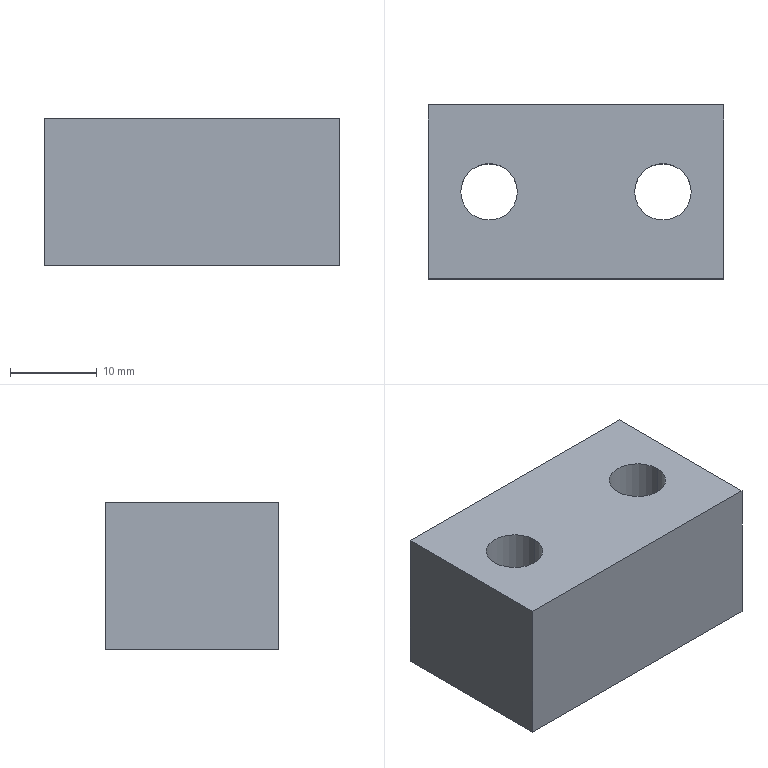Part | STEP file | push magnet seat spacer block 1 | 1 solid | 10 faces | box 34 x 20 x 17 mm | volume 10432 mm3 | plane 6 | cylinder 4 | commonest cylinder face diameters 6.5 x4
STEP:
#1=CARTESIAN_POINT('',(0.,0.,0.));
#2=DIRECTION('',(0.,0.,1.));
#3=DIRECTION('',(1.,0.,0.));
#4=AXIS2_PLACEMENT_3D('',#1,#2,#3);
#5=CARTESIAN_POINT('',(-13.25,0.,17.));
#6=VERTEX_POINT('',#5);
#7=CARTESIAN_POINT('',(-13.25,0.,0.));
#8=VERTEX_POINT('',#7);
#9=CARTESIAN_POINT('',(-13.25,0.,17.));
#10=DIRECTION('',(0.,0.,-1.));
#11=VECTOR('',#10,1.);
#12=LINE('',#9,#11);
#13=CARTESIAN_POINT('',(-10.,0.,17.));
#14=DIRECTION('',(0.,0.,-1.));
#15=DIRECTION('',(-1.,0.,0.));
#16=AXIS2_PLACEMENT_3D('',#13,#14,#15);
#17=CYLINDRICAL_SURFACE('',#16,3.25);
#18=CARTESIAN_POINT('',(6.283,0.));
#19=DIRECTION('',(0.,1.));
#20=VECTOR('',#19,1.);
#21=LINE('',#18,#20);
#22=(GEOMETRIC_REPRESENTATION_CONTEXT(2)PARAMETRIC_REPRESENTATION_CONTEXT()REPRESENTATION_CONTEXT('',''));
#23=DEFINITIONAL_REPRESENTATION('',(#21),#22);
#24=PCURVE('',#17,#23);
#25=CARTESIAN_POINT('',(-10.,0.,17.));
#26=DIRECTION('',(0.,0.,-1.));
#27=DIRECTION('',(-1.,0.,0.));
#28=AXIS2_PLACEMENT_3D('',#25,#26,#27);
#29=CYLINDRICAL_SURFACE('',#28,3.25);
#30=CARTESIAN_POINT('',(0.,0.));
#31=DIRECTION('',(0.,1.));
#32=VECTOR('',#31,1.);
#33=LINE('',#30,#32);
#34=(GEOMETRIC_REPRESENTATION_CONTEXT(2)PARAMETRIC_REPRESENTATION_CONTEXT()REPRESENTATION_CONTEXT('',''));
#35=DEFINITIONAL_REPRESENTATION('',(#33),#34);
#36=PCURVE('',#29,#35);
#37=SURFACE_CURVE('',#12,(#24,#36),.PCURVE_S1.);
#38=EDGE_CURVE('',#6,#8,#37,.T.);
#39=ORIENTED_EDGE('',*,*,#38,.T.);
#40=CARTESIAN_POINT('',(-6.75,0.,0.));
#41=VERTEX_POINT('',#40);
#42=CARTESIAN_POINT('',(-10.,0.,0.));
#43=DIRECTION('',(0.,0.,1.));
#44=DIRECTION('',(1.,0.,0.));
#45=AXIS2_PLACEMENT_3D('',#42,#43,#44);
#46=CIRCLE('',#45,3.25);
#47=CARTESIAN_POINT('',(9.425,17.));
#48=DIRECTION('',(-1.,0.));
#49=VECTOR('',#48,1.);
#50=LINE('',#47,#49);
#51=(GEOMETRIC_REPRESENTATION_CONTEXT(2)PARAMETRIC_REPRESENTATION_CONTEXT()REPRESENTATION_CONTEXT('',''));
#52=DEFINITIONAL_REPRESENTATION('',(#50),#51);
#53=PCURVE('',#17,#52);
#54=CARTESIAN_POINT('',(17.,-10.,0.));
#55=DIRECTION('',(0.,0.,1.));
#56=DIRECTION('',(1.,0.,0.));
#57=AXIS2_PLACEMENT_3D('',#54,#55,#56);
#58=PLANE('',#57);
#59=CARTESIAN_POINT('',(-27.,10.));
#60=DIRECTION('',(1.,0.));
#61=AXIS2_PLACEMENT_2D('',#59,#60);
#62=CIRCLE('',#61,3.25);
#63=(GEOMETRIC_REPRESENTATION_CONTEXT(2)PARAMETRIC_REPRESENTATION_CONTEXT()REPRESENTATION_CONTEXT('',''));
#64=DEFINITIONAL_REPRESENTATION('',(#62),#63);
#65=PCURVE('',#58,#64);
#66=SURFACE_CURVE('',#46,(#53,#65),.PCURVE_S1.);
#67=EDGE_CURVE('',#8,#41,#66,.T.);
#68=ORIENTED_EDGE('',*,*,#67,.T.);
#69=CARTESIAN_POINT('',(-6.75,0.,17.));
#70=VERTEX_POINT('',#69);
#71=CARTESIAN_POINT('',(-6.75,0.,17.));
#72=DIRECTION('',(0.,0.,-1.));
#73=VECTOR('',#72,1.);
#74=LINE('',#71,#73);
#75=CARTESIAN_POINT('',(3.142,0.));
#76=DIRECTION('',(0.,1.));
#77=VECTOR('',#76,1.);
#78=LINE('',#75,#77);
#79=(GEOMETRIC_REPRESENTATION_CONTEXT(2)PARAMETRIC_REPRESENTATION_CONTEXT()REPRESENTATION_CONTEXT('',''));
#80=DEFINITIONAL_REPRESENTATION('',(#78),#79);
#81=PCURVE('',#17,#80);
#82=CARTESIAN_POINT('',(3.142,0.));
#83=DIRECTION('',(0.,1.));
#84=VECTOR('',#83,1.);
#85=LINE('',#82,#84);
#86=(GEOMETRIC_REPRESENTATION_CONTEXT(2)PARAMETRIC_REPRESENTATION_CONTEXT()REPRESENTATION_CONTEXT('',''));
#87=DEFINITIONAL_REPRESENTATION('',(#85),#86);
#88=PCURVE('',#29,#87);
#89=SURFACE_CURVE('',#74,(#81,#88),.PCURVE_S1.);
#90=EDGE_CURVE('',#70,#41,#89,.T.);
#91=ORIENTED_EDGE('',*,*,#90,.F.);
#92=CARTESIAN_POINT('',(-10.,0.,17.));
#93=DIRECTION('',(0.,0.,1.));
#94=DIRECTION('',(1.,0.,0.));
#95=AXIS2_PLACEMENT_3D('',#92,#93,#94);
#96=CIRCLE('',#95,3.25);
#97=CARTESIAN_POINT('',(9.425,0.));
#98=DIRECTION('',(-1.,0.));
#99=VECTOR('',#98,1.);
#100=LINE('',#97,#99);
#101=(GEOMETRIC_REPRESENTATION_CONTEXT(2)PARAMETRIC_REPRESENTATION_CONTEXT()REPRESENTATION_CONTEXT('',''));
#102=DEFINITIONAL_REPRESENTATION('',(#100),#101);
#103=PCURVE('',#17,#102);
#104=CARTESIAN_POINT('',(17.,-10.,17.));
#105=DIRECTION('',(0.,0.,1.));
#106=DIRECTION('',(1.,0.,0.));
#107=AXIS2_PLACEMENT_3D('',#104,#105,#106);
#108=PLANE('',#107);
#109=CARTESIAN_POINT('',(-27.,10.));
#110=DIRECTION('',(1.,0.));
#111=AXIS2_PLACEMENT_2D('',#109,#110);
#112=CIRCLE('',#111,3.25);
#113=(GEOMETRIC_REPRESENTATION_CONTEXT(2)PARAMETRIC_REPRESENTATION_CONTEXT()REPRESENTATION_CONTEXT('',''));
#114=DEFINITIONAL_REPRESENTATION('',(#112),#113);
#115=PCURVE('',#108,#114);
#116=SURFACE_CURVE('',#96,(#103,#115),.PCURVE_S1.);
#117=EDGE_CURVE('',#6,#70,#116,.T.);
#118=ORIENTED_EDGE('',*,*,#117,.F.);
#119=EDGE_LOOP('',(#39,#68,#91,#118));
#120=FACE_BOUND('',#119,.F.);
#121=ADVANCED_FACE('',(#120),#17,.F.);
#122=CARTESIAN_POINT('',(6.75,0.,17.));
#123=VERTEX_POINT('',#122);
#124=CARTESIAN_POINT('',(6.75,0.,0.));
#125=VERTEX_POINT('',#124);
#126=CARTESIAN_POINT('',(6.75,0.,17.));
#127=DIRECTION('',(0.,0.,-1.));
#128=VECTOR('',#127,1.);
#129=LINE('',#126,#128);
#130=CARTESIAN_POINT('',(10.,0.,17.));
#131=DIRECTION('',(0.,0.,-1.));
#132=DIRECTION('',(-1.,0.,0.));
#133=AXIS2_PLACEMENT_3D('',#130,#131,#132);
#134=CYLINDRICAL_SURFACE('',#133,3.25);
#135=CARTESIAN_POINT('',(6.283,0.));
#136=DIRECTION('',(0.,1.));
#137=VECTOR('',#136,1.);
#138=LINE('',#135,#137);
#139=(GEOMETRIC_REPRESENTATION_CONTEXT(2)PARAMETRIC_REPRESENTATION_CONTEXT()REPRESENTATION_CONTEXT('',''));
#140=DEFINITIONAL_REPRESENTATION('',(#138),#139);
#141=PCURVE('',#134,#140);
#142=CARTESIAN_POINT('',(10.,0.,17.));
#143=DIRECTION('',(0.,0.,-1.));
#144=DIRECTION('',(-1.,0.,0.));
#145=AXIS2_PLACEMENT_3D('',#142,#143,#144);
#146=CYLINDRICAL_SURFACE('',#145,3.25);
#147=CARTESIAN_POINT('',(0.,0.));
#148=DIRECTION('',(0.,1.));
#149=VECTOR('',#148,1.);
#150=LINE('',#147,#149);
#151=(GEOMETRIC_REPRESENTATION_CONTEXT(2)PARAMETRIC_REPRESENTATION_CONTEXT()REPRESENTATION_CONTEXT('',''));
#152=DEFINITIONAL_REPRESENTATION('',(#150),#151);
#153=PCURVE('',#146,#152);
#154=SURFACE_CURVE('',#129,(#141,#153),.PCURVE_S1.);
#155=EDGE_CURVE('',#123,#125,#154,.T.);
#156=ORIENTED_EDGE('',*,*,#155,.T.);
#157=CARTESIAN_POINT('',(13.25,0.,0.));
#158=VERTEX_POINT('',#157);
#159=CARTESIAN_POINT('',(10.,0.,0.));
#160=DIRECTION('',(0.,0.,1.));
#161=DIRECTION('',(1.,0.,0.));
#162=AXIS2_PLACEMENT_3D('',#159,#160,#161);
#163=CIRCLE('',#162,3.25);
#164=CARTESIAN_POINT('',(9.425,17.));
#165=DIRECTION('',(-1.,0.));
#166=VECTOR('',#165,1.);
#167=LINE('',#164,#166);
#168=(GEOMETRIC_REPRESENTATION_CONTEXT(2)PARAMETRIC_REPRESENTATION_CONTEXT()REPRESENTATION_CONTEXT('',''));
#169=DEFINITIONAL_REPRESENTATION('',(#167),#168);
#170=PCURVE('',#134,#169);
#171=CARTESIAN_POINT('',(-7.,10.));
#172=DIRECTION('',(1.,0.));
#173=AXIS2_PLACEMENT_2D('',#171,#172);
#174=CIRCLE('',#173,3.25);
#175=(GEOMETRIC_REPRESENTATION_CONTEXT(2)PARAMETRIC_REPRESENTATION_CONTEXT()REPRESENTATION_CONTEXT('',''));
#176=DEFINITIONAL_REPRESENTATION('',(#174),#175);
#177=PCURVE('',#58,#176);
#178=SURFACE_CURVE('',#163,(#170,#177),.PCURVE_S1.);
#179=EDGE_CURVE('',#125,#158,#178,.T.);
#180=ORIENTED_EDGE('',*,*,#179,.T.);
#181=CARTESIAN_POINT('',(13.25,0.,17.));
#182=VERTEX_POINT('',#181);
#183=CARTESIAN_POINT('',(13.25,0.,17.));
#184=DIRECTION('',(0.,0.,-1.));
#185=VECTOR('',#184,1.);
#186=LINE('',#183,#185);
#187=CARTESIAN_POINT('',(3.142,0.));
#188=DIRECTION('',(0.,1.));
#189=VECTOR('',#188,1.);
#190=LINE('',#187,#189);
#191=(GEOMETRIC_REPRESENTATION_CONTEXT(2)PARAMETRIC_REPRESENTATION_CONTEXT()REPRESENTATION_CONTEXT('',''));
#192=DEFINITIONAL_REPRESENTATION('',(#190),#191);
#193=PCURVE('',#134,#192);
#194=CARTESIAN_POINT('',(3.142,0.));
#195=DIRECTION('',(0.,1.));
#196=VECTOR('',#195,1.);
#197=LINE('',#194,#196);
#198=(GEOMETRIC_REPRESENTATION_CONTEXT(2)PARAMETRIC_REPRESENTATION_CONTEXT()REPRESENTATION_CONTEXT('',''));
#199=DEFINITIONAL_REPRESENTATION('',(#197),#198);
#200=PCURVE('',#146,#199);
#201=SURFACE_CURVE('',#186,(#193,#200),.PCURVE_S1.);
#202=EDGE_CURVE('',#182,#158,#201,.T.);
#203=ORIENTED_EDGE('',*,*,#202,.F.);
#204=CARTESIAN_POINT('',(10.,0.,17.));
#205=DIRECTION('',(0.,0.,1.));
#206=DIRECTION('',(1.,0.,0.));
#207=AXIS2_PLACEMENT_3D('',#204,#205,#206);
#208=CIRCLE('',#207,3.25);
#209=CARTESIAN_POINT('',(9.425,0.));
#210=DIRECTION('',(-1.,0.));
#211=VECTOR('',#210,1.);
#212=LINE('',#209,#211);
#213=(GEOMETRIC_REPRESENTATION_CONTEXT(2)PARAMETRIC_REPRESENTATION_CONTEXT()REPRESENTATION_CONTEXT('',''));
#214=DEFINITIONAL_REPRESENTATION('',(#212),#213);
#215=PCURVE('',#134,#214);
#216=CARTESIAN_POINT('',(-7.,10.));
#217=DIRECTION('',(1.,0.));
#218=AXIS2_PLACEMENT_2D('',#216,#217);
#219=CIRCLE('',#218,3.25);
#220=(GEOMETRIC_REPRESENTATION_CONTEXT(2)PARAMETRIC_REPRESENTATION_CONTEXT()REPRESENTATION_CONTEXT('',''));
#221=DEFINITIONAL_REPRESENTATION('',(#219),#220);
#222=PCURVE('',#108,#221);
#223=SURFACE_CURVE('',#208,(#215,#222),.PCURVE_S1.);
#224=EDGE_CURVE('',#123,#182,#223,.T.);
#225=ORIENTED_EDGE('',*,*,#224,.F.);
#226=EDGE_LOOP('',(#156,#180,#203,#225));
#227=FACE_BOUND('',#226,.F.);
#228=ADVANCED_FACE('',(#227),#134,.F.);
#229=ORIENTED_EDGE('',*,*,#224,.F.);
#230=CARTESIAN_POINT('',(10.,0.,17.));
#231=DIRECTION('',(0.,0.,1.));
#232=DIRECTION('',(1.,0.,0.));
#233=AXIS2_PLACEMENT_3D('',#230,#231,#232);
#234=CIRCLE('',#233,3.25);
#235=CARTESIAN_POINT('',(-7.,10.));
#236=DIRECTION('',(1.,0.));
#237=AXIS2_PLACEMENT_2D('',#235,#236);
#238=CIRCLE('',#237,3.25);
#239=(GEOMETRIC_REPRESENTATION_CONTEXT(2)PARAMETRIC_REPRESENTATION_CONTEXT()REPRESENTATION_CONTEXT('',''));
#240=DEFINITIONAL_REPRESENTATION('',(#238),#239);
#241=PCURVE('',#108,#240);
#242=CARTESIAN_POINT('',(3.142,0.));
#243=DIRECTION('',(-1.,0.));
#244=VECTOR('',#243,1.);
#245=LINE('',#242,#244);
#246=(GEOMETRIC_REPRESENTATION_CONTEXT(2)PARAMETRIC_REPRESENTATION_CONTEXT()REPRESENTATION_CONTEXT('',''));
#247=DEFINITIONAL_REPRESENTATION('',(#245),#246);
#248=PCURVE('',#146,#247);
#249=SURFACE_CURVE('',#234,(#241,#248),.PCURVE_S1.);
#250=EDGE_CURVE('',#182,#123,#249,.T.);
#251=ORIENTED_EDGE('',*,*,#250,.F.);
#252=EDGE_LOOP('',(#229,#251));
#253=FACE_BOUND('',#252,.T.);
#254=CARTESIAN_POINT('',(17.,-10.,17.));
#255=VERTEX_POINT('',#254);
#256=CARTESIAN_POINT('',(17.,10.,17.));
#257=VERTEX_POINT('',#256);
#258=CARTESIAN_POINT('',(17.,10.,17.));
#259=DIRECTION('',(0.,1.,0.));
#260=VECTOR('',#259,1.);
#261=LINE('',#258,#260);
#262=CARTESIAN_POINT('',(0.,20.));
#263=DIRECTION('',(0.,1.));
#264=VECTOR('',#263,1.);
#265=LINE('',#262,#264);
#266=(GEOMETRIC_REPRESENTATION_CONTEXT(2)PARAMETRIC_REPRESENTATION_CONTEXT()REPRESENTATION_CONTEXT('',''));
#267=DEFINITIONAL_REPRESENTATION('',(#265),#266);
#268=PCURVE('',#108,#267);
#269=CARTESIAN_POINT('',(17.,10.,17.));
#270=DIRECTION('',(-1.,0.,0.));
#271=DIRECTION('',(0.,0.,1.));
#272=AXIS2_PLACEMENT_3D('',#269,#270,#271);
#273=PLANE('',#272);
#274=CARTESIAN_POINT('',(0.,0.));
#275=DIRECTION('',(0.,1.));
#276=VECTOR('',#275,1.);
#277=LINE('',#274,#276);
#278=(GEOMETRIC_REPRESENTATION_CONTEXT(2)PARAMETRIC_REPRESENTATION_CONTEXT()REPRESENTATION_CONTEXT('',''));
#279=DEFINITIONAL_REPRESENTATION('',(#277),#278);
#280=PCURVE('',#273,#279);
#281=SURFACE_CURVE('',#261,(#268,#280),.PCURVE_S1.);
#282=EDGE_CURVE('',#255,#257,#281,.T.);
#283=ORIENTED_EDGE('',*,*,#282,.T.);
#284=CARTESIAN_POINT('',(-17.,10.,17.));
#285=VERTEX_POINT('',#284);
#286=CARTESIAN_POINT('',(-17.,10.,17.));
#287=DIRECTION('',(-1.,0.,0.));
#288=VECTOR('',#287,1.);
#289=LINE('',#286,#288);
#290=CARTESIAN_POINT('',(-34.,20.));
#291=DIRECTION('',(-1.,0.));
#292=VECTOR('',#291,1.);
#293=LINE('',#290,#292);
#294=(GEOMETRIC_REPRESENTATION_CONTEXT(2)PARAMETRIC_REPRESENTATION_CONTEXT()REPRESENTATION_CONTEXT('',''));
#295=DEFINITIONAL_REPRESENTATION('',(#293),#294);
#296=PCURVE('',#108,#295);
#297=CARTESIAN_POINT('',(-17.,10.,17.));
#298=DIRECTION('',(0.,-1.,0.));
#299=DIRECTION('',(1.,0.,0.));
#300=AXIS2_PLACEMENT_3D('',#297,#298,#299);
#301=PLANE('',#300);
#302=CARTESIAN_POINT('',(0.,0.));
#303=DIRECTION('',(-1.,0.));
#304=VECTOR('',#303,1.);
#305=LINE('',#302,#304);
#306=(GEOMETRIC_REPRESENTATION_CONTEXT(2)PARAMETRIC_REPRESENTATION_CONTEXT()REPRESENTATION_CONTEXT('',''));
#307=DEFINITIONAL_REPRESENTATION('',(#305),#306);
#308=PCURVE('',#301,#307);
#309=SURFACE_CURVE('',#289,(#296,#308),.PCURVE_S1.);
#310=EDGE_CURVE('',#257,#285,#309,.T.);
#311=ORIENTED_EDGE('',*,*,#310,.T.);
#312=CARTESIAN_POINT('',(-17.,-10.,17.));
#313=VERTEX_POINT('',#312);
#314=CARTESIAN_POINT('',(-17.,10.,17.));
#315=DIRECTION('',(0.,-1.,0.));
#316=VECTOR('',#315,1.);
#317=LINE('',#314,#316);
#318=CARTESIAN_POINT('',(-34.,20.));
#319=DIRECTION('',(0.,-1.));
#320=VECTOR('',#319,1.);
#321=LINE('',#318,#320);
#322=(GEOMETRIC_REPRESENTATION_CONTEXT(2)PARAMETRIC_REPRESENTATION_CONTEXT()REPRESENTATION_CONTEXT('',''));
#323=DEFINITIONAL_REPRESENTATION('',(#321),#322);
#324=PCURVE('',#108,#323);
#325=CARTESIAN_POINT('',(-17.,10.,17.));
#326=DIRECTION('',(1.,0.,0.));
#327=DIRECTION('',(0.,0.,-1.));
#328=AXIS2_PLACEMENT_3D('',#325,#326,#327);
#329=PLANE('',#328);
#330=CARTESIAN_POINT('',(0.,0.));
#331=DIRECTION('',(0.,-1.));
#332=VECTOR('',#331,1.);
#333=LINE('',#330,#332);
#334=(GEOMETRIC_REPRESENTATION_CONTEXT(2)PARAMETRIC_REPRESENTATION_CONTEXT()REPRESENTATION_CONTEXT('',''));
#335=DEFINITIONAL_REPRESENTATION('',(#333),#334);
#336=PCURVE('',#329,#335);
#337=SURFACE_CURVE('',#317,(#324,#336),.PCURVE_S1.);
#338=EDGE_CURVE('',#285,#313,#337,.T.);
#339=ORIENTED_EDGE('',*,*,#338,.T.);
#340=CARTESIAN_POINT('',(-17.,-10.,17.));
#341=DIRECTION('',(1.,0.,0.));
#342=VECTOR('',#341,1.);
#343=LINE('',#340,#342);
#344=CARTESIAN_POINT('',(-34.,0.));
#345=DIRECTION('',(1.,0.));
#346=VECTOR('',#345,1.);
#347=LINE('',#344,#346);
#348=(GEOMETRIC_REPRESENTATION_CONTEXT(2)PARAMETRIC_REPRESENTATION_CONTEXT()REPRESENTATION_CONTEXT('',''));
#349=DEFINITIONAL_REPRESENTATION('',(#347),#348);
#350=PCURVE('',#108,#349);
#351=CARTESIAN_POINT('',(-17.,-10.,17.));
#352=DIRECTION('',(0.,1.,0.));
#353=DIRECTION('',(-1.,0.,0.));
#354=AXIS2_PLACEMENT_3D('',#351,#352,#353);
#355=PLANE('',#354);
#356=CARTESIAN_POINT('',(0.,0.));
#357=DIRECTION('',(-1.,0.));
#358=VECTOR('',#357,1.);
#359=LINE('',#356,#358);
#360=(GEOMETRIC_REPRESENTATION_CONTEXT(2)PARAMETRIC_REPRESENTATION_CONTEXT()REPRESENTATION_CONTEXT('',''));
#361=DEFINITIONAL_REPRESENTATION('',(#359),#360);
#362=PCURVE('',#355,#361);
#363=SURFACE_CURVE('',#343,(#350,#362),.PCURVE_S1.);
#364=EDGE_CURVE('',#313,#255,#363,.T.);
#365=ORIENTED_EDGE('',*,*,#364,.T.);
#366=EDGE_LOOP('',(#283,#311,#339,#365));
#367=FACE_BOUND('',#366,.T.);
#368=ORIENTED_EDGE('',*,*,#117,.F.);
#369=CARTESIAN_POINT('',(-10.,0.,17.));
#370=DIRECTION('',(0.,0.,1.));
#371=DIRECTION('',(1.,0.,0.));
#372=AXIS2_PLACEMENT_3D('',#369,#370,#371);
#373=CIRCLE('',#372,3.25);
#374=CARTESIAN_POINT('',(-27.,10.));
#375=DIRECTION('',(1.,0.));
#376=AXIS2_PLACEMENT_2D('',#374,#375);
#377=CIRCLE('',#376,3.25);
#378=(GEOMETRIC_REPRESENTATION_CONTEXT(2)PARAMETRIC_REPRESENTATION_CONTEXT()REPRESENTATION_CONTEXT('',''));
#379=DEFINITIONAL_REPRESENTATION('',(#377),#378);
#380=PCURVE('',#108,#379);
#381=CARTESIAN_POINT('',(3.142,0.));
#382=DIRECTION('',(-1.,0.));
#383=VECTOR('',#382,1.);
#384=LINE('',#381,#383);
#385=(GEOMETRIC_REPRESENTATION_CONTEXT(2)PARAMETRIC_REPRESENTATION_CONTEXT()REPRESENTATION_CONTEXT('',''));
#386=DEFINITIONAL_REPRESENTATION('',(#384),#385);
#387=PCURVE('',#29,#386);
#388=SURFACE_CURVE('',#373,(#380,#387),.PCURVE_S1.);
#389=EDGE_CURVE('',#70,#6,#388,.T.);
#390=ORIENTED_EDGE('',*,*,#389,.F.);
#391=EDGE_LOOP('',(#368,#390));
#392=FACE_BOUND('',#391,.T.);
#393=ADVANCED_FACE('',(#253,#367,#392),#108,.T.);
#394=ORIENTED_EDGE('',*,*,#179,.T.);
#395=CARTESIAN_POINT('',(10.,0.,0.));
#396=DIRECTION('',(0.,0.,1.));
#397=DIRECTION('',(1.,0.,0.));
#398=AXIS2_PLACEMENT_3D('',#395,#396,#397);
#399=CIRCLE('',#398,3.25);
#400=CARTESIAN_POINT('',(-7.,10.));
#401=DIRECTION('',(1.,0.));
#402=AXIS2_PLACEMENT_2D('',#400,#401);
#403=CIRCLE('',#402,3.25);
#404=(GEOMETRIC_REPRESENTATION_CONTEXT(2)PARAMETRIC_REPRESENTATION_CONTEXT()REPRESENTATION_CONTEXT('',''));
#405=DEFINITIONAL_REPRESENTATION('',(#403),#404);
#406=PCURVE('',#58,#405);
#407=CARTESIAN_POINT('',(3.142,17.));
#408=DIRECTION('',(-1.,0.));
#409=VECTOR('',#408,1.);
#410=LINE('',#407,#409);
#411=(GEOMETRIC_REPRESENTATION_CONTEXT(2)PARAMETRIC_REPRESENTATION_CONTEXT()REPRESENTATION_CONTEXT('',''));
#412=DEFINITIONAL_REPRESENTATION('',(#410),#411);
#413=PCURVE('',#146,#412);
#414=SURFACE_CURVE('',#399,(#406,#413),.PCURVE_S1.);
#415=EDGE_CURVE('',#158,#125,#414,.T.);
#416=ORIENTED_EDGE('',*,*,#415,.T.);
#417=EDGE_LOOP('',(#394,#416));
#418=FACE_BOUND('',#417,.T.);
#419=CARTESIAN_POINT('',(17.,-10.,0.));
#420=VERTEX_POINT('',#419);
#421=CARTESIAN_POINT('',(17.,10.,0.));
#422=VERTEX_POINT('',#421);
#423=CARTESIAN_POINT('',(17.,10.,0.));
#424=DIRECTION('',(0.,1.,0.));
#425=VECTOR('',#424,1.);
#426=LINE('',#423,#425);
#427=CARTESIAN_POINT('',(0.,20.));
#428=DIRECTION('',(0.,1.));
#429=VECTOR('',#428,1.);
#430=LINE('',#427,#429);
#431=(GEOMETRIC_REPRESENTATION_CONTEXT(2)PARAMETRIC_REPRESENTATION_CONTEXT()REPRESENTATION_CONTEXT('',''));
#432=DEFINITIONAL_REPRESENTATION('',(#430),#431);
#433=PCURVE('',#58,#432);
#434=CARTESIAN_POINT('',(-17.,0.));
#435=DIRECTION('',(0.,1.));
#436=VECTOR('',#435,1.);
#437=LINE('',#434,#436);
#438=(GEOMETRIC_REPRESENTATION_CONTEXT(2)PARAMETRIC_REPRESENTATION_CONTEXT()REPRESENTATION_CONTEXT('',''));
#439=DEFINITIONAL_REPRESENTATION('',(#437),#438);
#440=PCURVE('',#273,#439);
#441=SURFACE_CURVE('',#426,(#433,#440),.PCURVE_S1.);
#442=EDGE_CURVE('',#420,#422,#441,.T.);
#443=ORIENTED_EDGE('',*,*,#442,.F.);
#444=CARTESIAN_POINT('',(-17.,-10.,0.));
#445=VERTEX_POINT('',#444);
#446=CARTESIAN_POINT('',(-17.,-10.,0.));
#447=DIRECTION('',(1.,0.,0.));
#448=VECTOR('',#447,1.);
#449=LINE('',#446,#448);
#450=CARTESIAN_POINT('',(-34.,0.));
#451=DIRECTION('',(1.,0.));
#452=VECTOR('',#451,1.);
#453=LINE('',#450,#452);
#454=(GEOMETRIC_REPRESENTATION_CONTEXT(2)PARAMETRIC_REPRESENTATION_CONTEXT()REPRESENTATION_CONTEXT('',''));
#455=DEFINITIONAL_REPRESENTATION('',(#453),#454);
#456=PCURVE('',#58,#455);
#457=CARTESIAN_POINT('',(0.,-17.));
#458=DIRECTION('',(-1.,0.));
#459=VECTOR('',#458,1.);
#460=LINE('',#457,#459);
#461=(GEOMETRIC_REPRESENTATION_CONTEXT(2)PARAMETRIC_REPRESENTATION_CONTEXT()REPRESENTATION_CONTEXT('',''));
#462=DEFINITIONAL_REPRESENTATION('',(#460),#461);
#463=PCURVE('',#355,#462);
#464=SURFACE_CURVE('',#449,(#456,#463),.PCURVE_S1.);
#465=EDGE_CURVE('',#445,#420,#464,.T.);
#466=ORIENTED_EDGE('',*,*,#465,.F.);
#467=CARTESIAN_POINT('',(-17.,10.,0.));
#468=VERTEX_POINT('',#467);
#469=CARTESIAN_POINT('',(-17.,10.,0.));
#470=DIRECTION('',(0.,-1.,0.));
#471=VECTOR('',#470,1.);
#472=LINE('',#469,#471);
#473=CARTESIAN_POINT('',(-34.,20.));
#474=DIRECTION('',(0.,-1.));
#475=VECTOR('',#474,1.);
#476=LINE('',#473,#475);
#477=(GEOMETRIC_REPRESENTATION_CONTEXT(2)PARAMETRIC_REPRESENTATION_CONTEXT()REPRESENTATION_CONTEXT('',''));
#478=DEFINITIONAL_REPRESENTATION('',(#476),#477);
#479=PCURVE('',#58,#478);
#480=CARTESIAN_POINT('',(17.,0.));
#481=DIRECTION('',(0.,-1.));
#482=VECTOR('',#481,1.);
#483=LINE('',#480,#482);
#484=(GEOMETRIC_REPRESENTATION_CONTEXT(2)PARAMETRIC_REPRESENTATION_CONTEXT()REPRESENTATION_CONTEXT('',''));
#485=DEFINITIONAL_REPRESENTATION('',(#483),#484);
#486=PCURVE('',#329,#485);
#487=SURFACE_CURVE('',#472,(#479,#486),.PCURVE_S1.);
#488=EDGE_CURVE('',#468,#445,#487,.T.);
#489=ORIENTED_EDGE('',*,*,#488,.F.);
#490=CARTESIAN_POINT('',(-17.,10.,0.));
#491=DIRECTION('',(-1.,0.,0.));
#492=VECTOR('',#491,1.);
#493=LINE('',#490,#492);
#494=CARTESIAN_POINT('',(-34.,20.));
#495=DIRECTION('',(-1.,0.));
#496=VECTOR('',#495,1.);
#497=LINE('',#494,#496);
#498=(GEOMETRIC_REPRESENTATION_CONTEXT(2)PARAMETRIC_REPRESENTATION_CONTEXT()REPRESENTATION_CONTEXT('',''));
#499=DEFINITIONAL_REPRESENTATION('',(#497),#498);
#500=PCURVE('',#58,#499);
#501=CARTESIAN_POINT('',(0.,-17.));
#502=DIRECTION('',(-1.,0.));
#503=VECTOR('',#502,1.);
#504=LINE('',#501,#503);
#505=(GEOMETRIC_REPRESENTATION_CONTEXT(2)PARAMETRIC_REPRESENTATION_CONTEXT()REPRESENTATION_CONTEXT('',''));
#506=DEFINITIONAL_REPRESENTATION('',(#504),#505);
#507=PCURVE('',#301,#506);
#508=SURFACE_CURVE('',#493,(#500,#507),.PCURVE_S1.);
#509=EDGE_CURVE('',#422,#468,#508,.T.);
#510=ORIENTED_EDGE('',*,*,#509,.F.);
#511=EDGE_LOOP('',(#443,#466,#489,#510));
#512=FACE_BOUND('',#511,.T.);
#513=ORIENTED_EDGE('',*,*,#67,.T.);
#514=CARTESIAN_POINT('',(-10.,0.,0.));
#515=DIRECTION('',(0.,0.,1.));
#516=DIRECTION('',(1.,0.,0.));
#517=AXIS2_PLACEMENT_3D('',#514,#515,#516);
#518=CIRCLE('',#517,3.25);
#519=CARTESIAN_POINT('',(-27.,10.));
#520=DIRECTION('',(1.,0.));
#521=AXIS2_PLACEMENT_2D('',#519,#520);
#522=CIRCLE('',#521,3.25);
#523=(GEOMETRIC_REPRESENTATION_CONTEXT(2)PARAMETRIC_REPRESENTATION_CONTEXT()REPRESENTATION_CONTEXT('',''));
#524=DEFINITIONAL_REPRESENTATION('',(#522),#523);
#525=PCURVE('',#58,#524);
#526=CARTESIAN_POINT('',(3.142,17.));
#527=DIRECTION('',(-1.,0.));
#528=VECTOR('',#527,1.);
#529=LINE('',#526,#528);
#530=(GEOMETRIC_REPRESENTATION_CONTEXT(2)PARAMETRIC_REPRESENTATION_CONTEXT()REPRESENTATION_CONTEXT('',''));
#531=DEFINITIONAL_REPRESENTATION('',(#529),#530);
#532=PCURVE('',#29,#531);
#533=SURFACE_CURVE('',#518,(#525,#532),.PCURVE_S1.);
#534=EDGE_CURVE('',#41,#8,#533,.T.);
#535=ORIENTED_EDGE('',*,*,#534,.T.);
#536=EDGE_LOOP('',(#513,#535));
#537=FACE_BOUND('',#536,.T.);
#538=ADVANCED_FACE('',(#418,#512,#537),#58,.F.);
#539=ORIENTED_EDGE('',*,*,#442,.T.);
#540=CARTESIAN_POINT('',(17.,10.,17.));
#541=DIRECTION('',(0.,0.,-1.));
#542=VECTOR('',#541,1.);
#543=LINE('',#540,#542);
#544=CARTESIAN_POINT('',(0.,0.));
#545=DIRECTION('',(-1.,0.));
#546=VECTOR('',#545,1.);
#547=LINE('',#544,#546);
#548=(GEOMETRIC_REPRESENTATION_CONTEXT(2)PARAMETRIC_REPRESENTATION_CONTEXT()REPRESENTATION_CONTEXT('',''));
#549=DEFINITIONAL_REPRESENTATION('',(#547),#548);
#550=PCURVE('',#273,#549);
#551=CARTESIAN_POINT('',(34.,0.));
#552=DIRECTION('',(0.,-1.));
#553=VECTOR('',#552,1.);
#554=LINE('',#551,#553);
#555=(GEOMETRIC_REPRESENTATION_CONTEXT(2)PARAMETRIC_REPRESENTATION_CONTEXT()REPRESENTATION_CONTEXT('',''));
#556=DEFINITIONAL_REPRESENTATION('',(#554),#555);
#557=PCURVE('',#301,#556);
#558=SURFACE_CURVE('',#543,(#550,#557),.PCURVE_S1.);
#559=EDGE_CURVE('',#257,#422,#558,.T.);
#560=ORIENTED_EDGE('',*,*,#559,.F.);
#561=ORIENTED_EDGE('',*,*,#282,.F.);
#562=CARTESIAN_POINT('',(17.,-10.,17.));
#563=DIRECTION('',(0.,0.,-1.));
#564=VECTOR('',#563,1.);
#565=LINE('',#562,#564);
#566=CARTESIAN_POINT('',(0.,-20.));
#567=DIRECTION('',(-1.,0.));
#568=VECTOR('',#567,1.);
#569=LINE('',#566,#568);
#570=(GEOMETRIC_REPRESENTATION_CONTEXT(2)PARAMETRIC_REPRESENTATION_CONTEXT()REPRESENTATION_CONTEXT('',''));
#571=DEFINITIONAL_REPRESENTATION('',(#569),#570);
#572=PCURVE('',#273,#571);
#573=CARTESIAN_POINT('',(-34.,0.));
#574=DIRECTION('',(0.,-1.));
#575=VECTOR('',#574,1.);
#576=LINE('',#573,#575);
#577=(GEOMETRIC_REPRESENTATION_CONTEXT(2)PARAMETRIC_REPRESENTATION_CONTEXT()REPRESENTATION_CONTEXT('',''));
#578=DEFINITIONAL_REPRESENTATION('',(#576),#577);
#579=PCURVE('',#355,#578);
#580=SURFACE_CURVE('',#565,(#572,#579),.PCURVE_S1.);
#581=EDGE_CURVE('',#255,#420,#580,.T.);
#582=ORIENTED_EDGE('',*,*,#581,.T.);
#583=EDGE_LOOP('',(#539,#560,#561,#582));
#584=FACE_BOUND('',#583,.T.);
#585=ADVANCED_FACE('',(#584),#273,.F.);
#586=ORIENTED_EDGE('',*,*,#509,.T.);
#587=CARTESIAN_POINT('',(-17.,10.,17.));
#588=DIRECTION('',(0.,0.,-1.));
#589=VECTOR('',#588,1.);
#590=LINE('',#587,#589);
#591=CARTESIAN_POINT('',(0.,0.));
#592=DIRECTION('',(0.,-1.));
#593=VECTOR('',#592,1.);
#594=LINE('',#591,#593);
#595=(GEOMETRIC_REPRESENTATION_CONTEXT(2)PARAMETRIC_REPRESENTATION_CONTEXT()REPRESENTATION_CONTEXT('',''));
#596=DEFINITIONAL_REPRESENTATION('',(#594),#595);
#597=PCURVE('',#301,#596);
#598=CARTESIAN_POINT('',(0.,0.));
#599=DIRECTION('',(1.,0.));
#600=VECTOR('',#599,1.);
#601=LINE('',#598,#600);
#602=(GEOMETRIC_REPRESENTATION_CONTEXT(2)PARAMETRIC_REPRESENTATION_CONTEXT()REPRESENTATION_CONTEXT('',''));
#603=DEFINITIONAL_REPRESENTATION('',(#601),#602);
#604=PCURVE('',#329,#603);
#605=SURFACE_CURVE('',#590,(#597,#604),.PCURVE_S1.);
#606=EDGE_CURVE('',#285,#468,#605,.T.);
#607=ORIENTED_EDGE('',*,*,#606,.F.);
#608=ORIENTED_EDGE('',*,*,#310,.F.);
#609=ORIENTED_EDGE('',*,*,#559,.T.);
#610=EDGE_LOOP('',(#586,#607,#608,#609));
#611=FACE_BOUND('',#610,.T.);
#612=ADVANCED_FACE('',(#611),#301,.F.);
#613=ORIENTED_EDGE('',*,*,#488,.T.);
#614=CARTESIAN_POINT('',(-17.,-10.,17.));
#615=DIRECTION('',(0.,0.,-1.));
#616=VECTOR('',#615,1.);
#617=LINE('',#614,#616);
#618=CARTESIAN_POINT('',(0.,-20.));
#619=DIRECTION('',(1.,0.));
#620=VECTOR('',#619,1.);
#621=LINE('',#618,#620);
#622=(GEOMETRIC_REPRESENTATION_CONTEXT(2)PARAMETRIC_REPRESENTATION_CONTEXT()REPRESENTATION_CONTEXT('',''));
#623=DEFINITIONAL_REPRESENTATION('',(#621),#622);
#624=PCURVE('',#329,#623);
#625=CARTESIAN_POINT('',(0.,0.));
#626=DIRECTION('',(0.,-1.));
#627=VECTOR('',#626,1.);
#628=LINE('',#625,#627);
#629=(GEOMETRIC_REPRESENTATION_CONTEXT(2)PARAMETRIC_REPRESENTATION_CONTEXT()REPRESENTATION_CONTEXT('',''));
#630=DEFINITIONAL_REPRESENTATION('',(#628),#629);
#631=PCURVE('',#355,#630);
#632=SURFACE_CURVE('',#617,(#624,#631),.PCURVE_S1.);
#633=EDGE_CURVE('',#313,#445,#632,.T.);
#634=ORIENTED_EDGE('',*,*,#633,.F.);
#635=ORIENTED_EDGE('',*,*,#338,.F.);
#636=ORIENTED_EDGE('',*,*,#606,.T.);
#637=EDGE_LOOP('',(#613,#634,#635,#636));
#638=FACE_BOUND('',#637,.T.);
#639=ADVANCED_FACE('',(#638),#329,.F.);
#640=ORIENTED_EDGE('',*,*,#465,.T.);
#641=ORIENTED_EDGE('',*,*,#581,.F.);
#642=ORIENTED_EDGE('',*,*,#364,.F.);
#643=ORIENTED_EDGE('',*,*,#633,.T.);
#644=EDGE_LOOP('',(#640,#641,#642,#643));
#645=FACE_BOUND('',#644,.T.);
#646=ADVANCED_FACE('',(#645),#355,.F.);
#647=ORIENTED_EDGE('',*,*,#415,.T.);
#648=ORIENTED_EDGE('',*,*,#155,.F.);
#649=ORIENTED_EDGE('',*,*,#250,.F.);
#650=ORIENTED_EDGE('',*,*,#202,.T.);
#651=EDGE_LOOP('',(#647,#648,#649,#650));
#652=FACE_BOUND('',#651,.F.);
#653=ADVANCED_FACE('',(#652),#146,.F.);
#654=ORIENTED_EDGE('',*,*,#534,.T.);
#655=ORIENTED_EDGE('',*,*,#38,.F.);
#656=ORIENTED_EDGE('',*,*,#389,.F.);
#657=ORIENTED_EDGE('',*,*,#90,.T.);
#658=EDGE_LOOP('',(#654,#655,#656,#657));
#659=FACE_BOUND('',#658,.F.);
#660=ADVANCED_FACE('',(#659),#29,.F.);
#661=CLOSED_SHELL('',(#121,#228,#393,#538,#585,#612,#639,#646,#653,#660));
#662=MANIFOLD_SOLID_BREP('',#661);
#663=(LENGTH_UNIT()NAMED_UNIT(*)SI_UNIT(.MILLI.,.METRE.));
#664=UNCERTAINTY_MEASURE_WITH_UNIT(LENGTH_MEASURE(0.0000001),#663,'','');
#665=(NAMED_UNIT(*)PLANE_ANGLE_UNIT()SI_UNIT($,.RADIAN.));
#666=(NAMED_UNIT(*)SI_UNIT($,.STERADIAN.)SOLID_ANGLE_UNIT());
#667=(GEOMETRIC_REPRESENTATION_CONTEXT(3)GLOBAL_UNCERTAINTY_ASSIGNED_CONTEXT((#664))GLOBAL_UNIT_ASSIGNED_CONTEXT((#663,#665,#666))REPRESENTATION_CONTEXT('',''));
#668=ADVANCED_BREP_SHAPE_REPRESENTATION('',(#4,#662),#667);